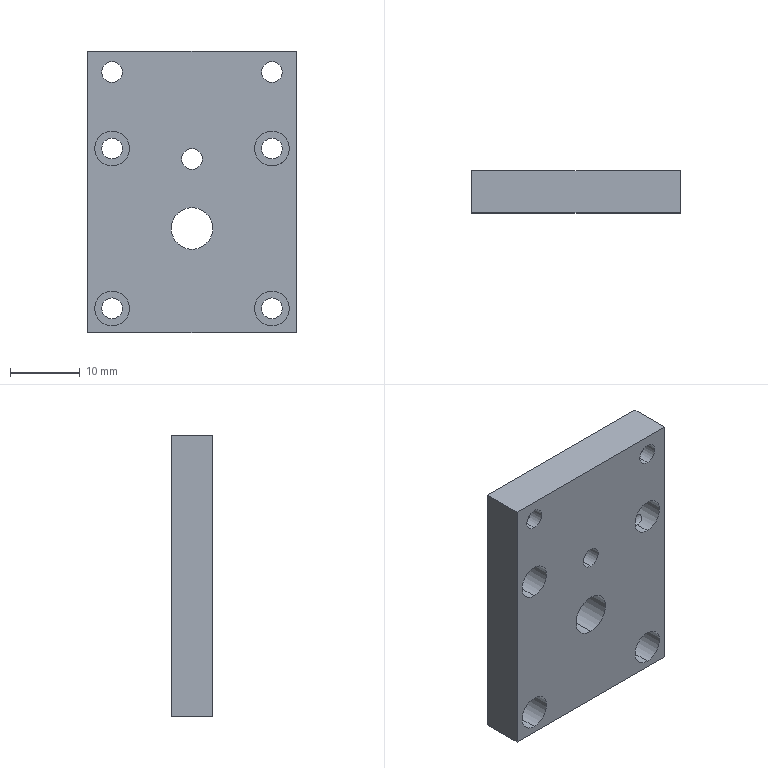Part | SolidWorks | features Cut 3, ICE 3, FlatPattern 1, HoleWzd 1, SMBaseFlange 1, SheetMetal 1 | 1 solid | 48 faces | box 30 x 6 x 40.5 mm | volume 6447 mm3 | cylinder 32 | plane 12 | cone 4 | commonest cylinder face diameters 3 x14 5 x12 2.5 x4 6 x2
STEP:
#1=CARTESIAN_POINT('',(6.749,-3.,3.));
#2=VERTEX_POINT('',#1);
#3=CARTESIAN_POINT('',(7.5,-3.,1.75));
#4=VERTEX_POINT('',#3);
#5=CARTESIAN_POINT('',(7.5,-3.,1.75));
#6=DIRECTION('',(0.515,0.,-0.8572));
#7=VECTOR('',#6,1000.);
#8=LINE('',#5,#7);
#9=EDGE_CURVE('',#2,#4,#8,.T.);
#10=ORIENTED_EDGE('',*,*,#9,.F.);
#11=CARTESIAN_POINT('',(7.5,-3.,4.25));
#12=VERTEX_POINT('',#11);
#13=CARTESIAN_POINT('',(7.5,-3.,4.25));
#14=DIRECTION('',(0.515,0.,0.8572));
#15=VECTOR('',#14,1000.);
#16=LINE('',#13,#15);
#17=EDGE_CURVE('',#2,#12,#16,.T.);
#18=ORIENTED_EDGE('',*,*,#17,.T.);
#19=CARTESIAN_POINT('',(7.5,-3.,3.));
#20=DIRECTION('',(1.,0.,0.));
#21=DIRECTION('',(0.,0.,-1.));
#22=AXIS2_PLACEMENT_3D('',#19,#20,#21);
#23=CIRCLE('',#22,1.25);
#24=EDGE_CURVE('',#12,#4,#23,.T.);
#25=ORIENTED_EDGE('',*,*,#24,.T.);
#26=EDGE_LOOP('',(#10,#18,#25));
#27=FACE_OUTER_BOUND('',#26,.T.);
#28=CARTESIAN_POINT('',(7.5,-3.,3.));
#29=DIRECTION('',(1.,0.,0.));
#30=DIRECTION('',(0.,0.,-1.));
#31=AXIS2_PLACEMENT_3D('',#28,#29,#30);
#32=CONICAL_SURFACE('',#31,1.25,1.03);
#33=ADVANCED_FACE('',(#27),#32,.F.);
#34=ORIENTED_EDGE('',*,*,#24,.F.);
#35=CARTESIAN_POINT('',(10.,-3.,4.25));
#36=VERTEX_POINT('',#35);
#37=CARTESIAN_POINT('',(15.,-3.,4.25));
#38=DIRECTION('',(1.,0.,0.));
#39=VECTOR('',#38,1000.);
#40=LINE('',#37,#39);
#41=EDGE_CURVE('',#12,#36,#40,.T.);
#42=ORIENTED_EDGE('',*,*,#41,.T.);
#43=CARTESIAN_POINT('',(11.5,-4.,3.75));
#44=VERTEX_POINT('',#43);
#45=CARTESIAN_POINT('',(11.5,-4.,3.75));
#46=CARTESIAN_POINT('',(11.325,-4.,3.75));
#47=CARTESIAN_POINT('',(11.15,-3.987,3.769));
#48=CARTESIAN_POINT('',(10.815,-3.927,3.839));
#49=CARTESIAN_POINT('',(10.651,-3.88,3.893));
#50=CARTESIAN_POINT('',(10.362,-3.731,4.019));
#51=CARTESIAN_POINT('',(10.233,-3.627,4.092));
#52=CARTESIAN_POINT('',(10.051,-3.348,4.21));
#53=CARTESIAN_POINT('',(10.,-3.177,4.25));
#54=CARTESIAN_POINT('',(10.,-3.,4.25));
#55=B_SPLINE_CURVE_WITH_KNOTS('',3,(#45,#46,#47,#48,#49,#50,#51,#52,#53,#54),.UNSPECIFIED.,.F.,.F.,(4,2,2,2,4),(0.004168,0.004689,0.00521,0.005731,0.006252),.UNSPECIFIED.);
#56=EDGE_CURVE('',#44,#36,#55,.T.);
#57=ORIENTED_EDGE('',*,*,#56,.F.);
#58=CARTESIAN_POINT('',(13.,-3.,4.25));
#59=VERTEX_POINT('',#58);
#60=CARTESIAN_POINT('',(13.,-3.,4.25));
#61=CARTESIAN_POINT('',(13.,-3.176,4.25));
#62=CARTESIAN_POINT('',(12.949,-3.349,4.21));
#63=CARTESIAN_POINT('',(12.813,-3.557,4.122));
#64=CARTESIAN_POINT('',(12.758,-3.618,4.088));
#65=CARTESIAN_POINT('',(12.634,-3.724,4.021));
#66=CARTESIAN_POINT('',(12.567,-3.768,3.988));
#67=CARTESIAN_POINT('',(12.349,-3.88,3.893));
#68=CARTESIAN_POINT('',(12.187,-3.927,3.84));
#69=CARTESIAN_POINT('',(11.85,-3.987,3.769));
#70=CARTESIAN_POINT('',(11.675,-4.,3.75));
#71=CARTESIAN_POINT('',(11.5,-4.,3.75));
#72=B_SPLINE_CURVE_WITH_KNOTS('',3,(#60,#61,#62,#63,#64,#65,#66,#67,#68,#69,#70,#71),.UNSPECIFIED.,.F.,.F.,(4,2,2,2,2,4),(0.002085,0.002606,0.002866,0.003126,0.003647,0.004168),.UNSPECIFIED.);
#73=EDGE_CURVE('',#59,#44,#72,.T.);
#74=ORIENTED_EDGE('',*,*,#73,.F.);
#75=CARTESIAN_POINT('',(15.,-3.,4.25));
#76=VERTEX_POINT('',#75);
#77=CARTESIAN_POINT('',(15.,-3.,4.25));
#78=DIRECTION('',(1.,0.,0.));
#79=VECTOR('',#78,1000.);
#80=LINE('',#77,#79);
#81=EDGE_CURVE('',#59,#76,#80,.T.);
#82=ORIENTED_EDGE('',*,*,#81,.T.);
#83=CARTESIAN_POINT('',(15.,-3.,1.75));
#84=VERTEX_POINT('',#83);
#85=CARTESIAN_POINT('',(15.,-3.,3.));
#86=DIRECTION('',(1.,0.,0.));
#87=DIRECTION('',(0.,0.,-1.));
#88=AXIS2_PLACEMENT_3D('',#85,#86,#87);
#89=CIRCLE('',#88,1.25);
#90=EDGE_CURVE('',#76,#84,#89,.T.);
#91=ORIENTED_EDGE('',*,*,#90,.T.);
#92=CARTESIAN_POINT('',(15.,-3.,1.75));
#93=DIRECTION('',(1.,0.,0.));
#94=VECTOR('',#93,1000.);
#95=LINE('',#92,#94);
#96=EDGE_CURVE('',#4,#84,#95,.T.);
#97=ORIENTED_EDGE('',*,*,#96,.F.);
#98=EDGE_LOOP('',(#34,#42,#57,#74,#82,#91,#97));
#99=FACE_OUTER_BOUND('',#98,.T.);
#100=CARTESIAN_POINT('',(15.,-3.,3.));
#101=DIRECTION('',(1.,0.,0.));
#102=DIRECTION('',(0.,0.,-1.));
#103=AXIS2_PLACEMENT_3D('',#100,#101,#102);
#104=CYLINDRICAL_SURFACE('',#103,1.25);
#105=ADVANCED_FACE('',(#99),#104,.F.);
#106=CARTESIAN_POINT('',(7.5,-3.,-5.25));
#107=VERTEX_POINT('',#106);
#108=CARTESIAN_POINT('',(7.5,-3.,-7.75));
#109=VERTEX_POINT('',#108);
#110=CARTESIAN_POINT('',(7.5,-3.,-6.5));
#111=DIRECTION('',(1.,0.,0.));
#112=DIRECTION('',(0.,0.,-1.));
#113=AXIS2_PLACEMENT_3D('',#110,#111,#112);
#114=CIRCLE('',#113,1.25);
#115=EDGE_CURVE('',#107,#109,#114,.T.);
#116=ORIENTED_EDGE('',*,*,#115,.F.);
#117=CARTESIAN_POINT('',(15.,-3.,-5.25));
#118=VERTEX_POINT('',#117);
#119=CARTESIAN_POINT('',(15.,-3.,-5.25));
#120=DIRECTION('',(1.,0.,0.));
#121=VECTOR('',#120,1000.);
#122=LINE('',#119,#121);
#123=EDGE_CURVE('',#107,#118,#122,.T.);
#124=ORIENTED_EDGE('',*,*,#123,.T.);
#125=CARTESIAN_POINT('',(15.,-3.,-7.75));
#126=VERTEX_POINT('',#125);
#127=CARTESIAN_POINT('',(15.,-3.,-6.5));
#128=DIRECTION('',(1.,0.,0.));
#129=DIRECTION('',(0.,0.,-1.));
#130=AXIS2_PLACEMENT_3D('',#127,#128,#129);
#131=CIRCLE('',#130,1.25);
#132=EDGE_CURVE('',#118,#126,#131,.T.);
#133=ORIENTED_EDGE('',*,*,#132,.T.);
#134=CARTESIAN_POINT('',(15.,-3.,-7.75));
#135=DIRECTION('',(1.,0.,0.));
#136=VECTOR('',#135,1000.);
#137=LINE('',#134,#136);
#138=EDGE_CURVE('',#109,#126,#137,.T.);
#139=ORIENTED_EDGE('',*,*,#138,.F.);
#140=EDGE_LOOP('',(#116,#124,#133,#139));
#141=FACE_OUTER_BOUND('',#140,.T.);
#142=CARTESIAN_POINT('',(15.,-3.,-6.5));
#143=DIRECTION('',(1.,0.,0.));
#144=DIRECTION('',(0.,0.,-1.));
#145=AXIS2_PLACEMENT_3D('',#142,#143,#144);
#146=CYLINDRICAL_SURFACE('',#145,1.25);
#147=ADVANCED_FACE('',(#141),#146,.F.);
#148=CARTESIAN_POINT('',(6.749,-3.,-6.5));
#149=VERTEX_POINT('',#148);
#150=CARTESIAN_POINT('',(7.5,-3.,-7.75));
#151=DIRECTION('',(0.515,0.,-0.8572));
#152=VECTOR('',#151,1000.);
#153=LINE('',#150,#152);
#154=EDGE_CURVE('',#149,#109,#153,.T.);
#155=ORIENTED_EDGE('',*,*,#154,.F.);
#156=CARTESIAN_POINT('',(7.5,-3.,-5.25));
#157=DIRECTION('',(0.515,0.,0.8572));
#158=VECTOR('',#157,1000.);
#159=LINE('',#156,#158);
#160=EDGE_CURVE('',#149,#107,#159,.T.);
#161=ORIENTED_EDGE('',*,*,#160,.T.);
#162=ORIENTED_EDGE('',*,*,#115,.T.);
#163=EDGE_LOOP('',(#155,#161,#162));
#164=FACE_OUTER_BOUND('',#163,.T.);
#165=CARTESIAN_POINT('',(7.5,-3.,-6.5));
#166=DIRECTION('',(1.,0.,0.));
#167=DIRECTION('',(0.,0.,-1.));
#168=AXIS2_PLACEMENT_3D('',#165,#166,#167);
#169=CONICAL_SURFACE('',#168,1.25,1.03);
#170=ADVANCED_FACE('',(#164),#169,.F.);
#171=CARTESIAN_POINT('',(11.5,-4.,14.75));
#172=VERTEX_POINT('',#171);
#173=CARTESIAN_POINT('',(11.5,-4.,19.75));
#174=VERTEX_POINT('',#173);
#175=CARTESIAN_POINT('',(11.5,-4.,17.25));
#176=DIRECTION('',(0.,1.,0.));
#177=DIRECTION('',(0.,0.,1.));
#178=AXIS2_PLACEMENT_3D('',#175,#176,#177);
#179=CIRCLE('',#178,2.5);
#180=EDGE_CURVE('',#172,#174,#179,.T.);
#181=ORIENTED_EDGE('',*,*,#180,.F.);
#182=CARTESIAN_POINT('',(11.5,0.,14.75));
#183=VERTEX_POINT('',#182);
#184=CARTESIAN_POINT('',(11.5,-4.,14.75));
#185=DIRECTION('',(0.,1.,0.));
#186=VECTOR('',#185,1000.);
#187=LINE('',#184,#186);
#188=EDGE_CURVE('',#172,#183,#187,.T.);
#189=ORIENTED_EDGE('',*,*,#188,.T.);
#190=CARTESIAN_POINT('',(11.5,0.,19.75));
#191=VERTEX_POINT('',#190);
#192=CARTESIAN_POINT('',(11.5,0.,17.25));
#193=DIRECTION('',(0.,1.,0.));
#194=DIRECTION('',(0.,0.,1.));
#195=AXIS2_PLACEMENT_3D('',#192,#193,#194);
#196=CIRCLE('',#195,2.5);
#197=EDGE_CURVE('',#183,#191,#196,.T.);
#198=ORIENTED_EDGE('',*,*,#197,.T.);
#199=CARTESIAN_POINT('',(11.5,-4.,19.75));
#200=DIRECTION('',(0.,1.,0.));
#201=VECTOR('',#200,1000.);
#202=LINE('',#199,#201);
#203=EDGE_CURVE('',#174,#191,#202,.T.);
#204=ORIENTED_EDGE('',*,*,#203,.F.);
#205=EDGE_LOOP('',(#181,#189,#198,#204));
#206=FACE_OUTER_BOUND('',#205,.T.);
#207=CARTESIAN_POINT('',(11.5,-4.,17.25));
#208=DIRECTION('',(0.,1.,0.));
#209=DIRECTION('',(0.,0.,1.));
#210=AXIS2_PLACEMENT_3D('',#207,#208,#209);
#211=CYLINDRICAL_SURFACE('',#210,2.5);
#212=ADVANCED_FACE('',(#206),#211,.F.);
#213=CARTESIAN_POINT('',(-11.5,-4.,14.75));
#214=VERTEX_POINT('',#213);
#215=CARTESIAN_POINT('',(-11.5,-4.,19.75));
#216=VERTEX_POINT('',#215);
#217=CARTESIAN_POINT('',(-11.5,-4.,17.25));
#218=DIRECTION('',(0.,1.,0.));
#219=DIRECTION('',(0.,0.,1.));
#220=AXIS2_PLACEMENT_3D('',#217,#218,#219);
#221=CIRCLE('',#220,2.5);
#222=EDGE_CURVE('',#214,#216,#221,.T.);
#223=ORIENTED_EDGE('',*,*,#222,.F.);
#224=CARTESIAN_POINT('',(-11.5,0.,14.75));
#225=VERTEX_POINT('',#224);
#226=CARTESIAN_POINT('',(-11.5,-4.,14.75));
#227=DIRECTION('',(0.,1.,0.));
#228=VECTOR('',#227,1000.);
#229=LINE('',#226,#228);
#230=EDGE_CURVE('',#214,#225,#229,.T.);
#231=ORIENTED_EDGE('',*,*,#230,.T.);
#232=CARTESIAN_POINT('',(-11.5,0.,19.75));
#233=VERTEX_POINT('',#232);
#234=CARTESIAN_POINT('',(-11.5,0.,17.25));
#235=DIRECTION('',(0.,1.,0.));
#236=DIRECTION('',(0.,0.,1.));
#237=AXIS2_PLACEMENT_3D('',#234,#235,#236);
#238=CIRCLE('',#237,2.5);
#239=EDGE_CURVE('',#225,#233,#238,.T.);
#240=ORIENTED_EDGE('',*,*,#239,.T.);
#241=CARTESIAN_POINT('',(-11.5,-4.,19.75));
#242=DIRECTION('',(0.,1.,0.));
#243=VECTOR('',#242,1000.);
#244=LINE('',#241,#243);
#245=EDGE_CURVE('',#216,#233,#244,.T.);
#246=ORIENTED_EDGE('',*,*,#245,.F.);
#247=EDGE_LOOP('',(#223,#231,#240,#246));
#248=FACE_OUTER_BOUND('',#247,.T.);
#249=CARTESIAN_POINT('',(-11.5,-4.,17.25));
#250=DIRECTION('',(0.,1.,0.));
#251=DIRECTION('',(0.,0.,1.));
#252=AXIS2_PLACEMENT_3D('',#249,#250,#251);
#253=CYLINDRICAL_SURFACE('',#252,2.5);
#254=ADVANCED_FACE('',(#248),#253,.F.);
#255=CARTESIAN_POINT('',(11.5,-2.,-14.25));
#256=VERTEX_POINT('',#255);
#257=CARTESIAN_POINT('',(11.5,-2.,-19.25));
#258=VERTEX_POINT('',#257);
#259=CARTESIAN_POINT('',(11.5,-2.,-16.75));
#260=DIRECTION('',(0.,-1.,0.));
#261=DIRECTION('',(0.,0.,-1.));
#262=AXIS2_PLACEMENT_3D('',#259,#260,#261);
#263=CIRCLE('',#262,2.5);
#264=EDGE_CURVE('',#256,#258,#263,.T.);
#265=ORIENTED_EDGE('',*,*,#264,.F.);
#266=CARTESIAN_POINT('',(11.5,-6.,-14.25));
#267=VERTEX_POINT('',#266);
#268=CARTESIAN_POINT('',(11.5,-2.,-14.25));
#269=DIRECTION('',(0.,-1.,0.));
#270=VECTOR('',#269,1000.);
#271=LINE('',#268,#270);
#272=EDGE_CURVE('',#256,#267,#271,.T.);
#273=ORIENTED_EDGE('',*,*,#272,.T.);
#274=CARTESIAN_POINT('',(11.5,-6.,-19.25));
#275=VERTEX_POINT('',#274);
#276=CARTESIAN_POINT('',(11.5,-6.,-16.75));
#277=DIRECTION('',(0.,-1.,0.));
#278=DIRECTION('',(0.,0.,-1.));
#279=AXIS2_PLACEMENT_3D('',#276,#277,#278);
#280=CIRCLE('',#279,2.5);
#281=EDGE_CURVE('',#267,#275,#280,.T.);
#282=ORIENTED_EDGE('',*,*,#281,.T.);
#283=CARTESIAN_POINT('',(11.5,-2.,-19.25));
#284=DIRECTION('',(0.,-1.,0.));
#285=VECTOR('',#284,1000.);
#286=LINE('',#283,#285);
#287=EDGE_CURVE('',#258,#275,#286,.T.);
#288=ORIENTED_EDGE('',*,*,#287,.F.);
#289=EDGE_LOOP('',(#265,#273,#282,#288));
#290=FACE_OUTER_BOUND('',#289,.T.);
#291=CARTESIAN_POINT('',(11.5,-2.,-16.75));
#292=DIRECTION('',(0.,-1.,0.));
#293=DIRECTION('',(0.,0.,-1.));
#294=AXIS2_PLACEMENT_3D('',#291,#292,#293);
#295=CYLINDRICAL_SURFACE('',#294,2.5);
#296=ADVANCED_FACE('',(#290),#295,.F.);
#297=CARTESIAN_POINT('',(11.5,-2.,8.75));
#298=VERTEX_POINT('',#297);
#299=CARTESIAN_POINT('',(11.5,-2.,3.75));
#300=VERTEX_POINT('',#299);
#301=CARTESIAN_POINT('',(11.5,-2.,6.25));
#302=DIRECTION('',(0.,-1.,0.));
#303=DIRECTION('',(0.,0.,-1.));
#304=AXIS2_PLACEMENT_3D('',#301,#302,#303);
#305=CIRCLE('',#304,2.5);
#306=EDGE_CURVE('',#298,#300,#305,.T.);
#307=ORIENTED_EDGE('',*,*,#306,.F.);
#308=CARTESIAN_POINT('',(11.5,-6.,8.75));
#309=VERTEX_POINT('',#308);
#310=CARTESIAN_POINT('',(11.5,-2.,8.75));
#311=DIRECTION('',(0.,-1.,0.));
#312=VECTOR('',#311,1000.);
#313=LINE('',#310,#312);
#314=EDGE_CURVE('',#298,#309,#313,.T.);
#315=ORIENTED_EDGE('',*,*,#314,.T.);
#316=CARTESIAN_POINT('',(11.5,-6.,3.75));
#317=VERTEX_POINT('',#316);
#318=CARTESIAN_POINT('',(11.5,-6.,6.25));
#319=DIRECTION('',(0.,-1.,0.));
#320=DIRECTION('',(0.,0.,-1.));
#321=AXIS2_PLACEMENT_3D('',#318,#319,#320);
#322=CIRCLE('',#321,2.5);
#323=EDGE_CURVE('',#309,#317,#322,.T.);
#324=ORIENTED_EDGE('',*,*,#323,.T.);
#325=CARTESIAN_POINT('',(11.5,-2.,3.75));
#326=DIRECTION('',(0.,-1.,0.));
#327=VECTOR('',#326,1000.);
#328=LINE('',#325,#327);
#329=EDGE_CURVE('',#44,#317,#328,.T.);
#330=ORIENTED_EDGE('',*,*,#329,.F.);
#331=ORIENTED_EDGE('',*,*,#56,.T.);
#332=CARTESIAN_POINT('',(10.,-3.,4.25));
#333=CARTESIAN_POINT('',(10.,-2.823,4.25));
#334=CARTESIAN_POINT('',(10.051,-2.652,4.21));
#335=CARTESIAN_POINT('',(10.233,-2.373,4.092));
#336=CARTESIAN_POINT('',(10.361,-2.269,4.019));
#337=CARTESIAN_POINT('',(10.65,-2.121,3.894));
#338=CARTESIAN_POINT('',(10.813,-2.073,3.84));
#339=CARTESIAN_POINT('',(11.148,-2.013,3.769));
#340=CARTESIAN_POINT('',(11.324,-2.,3.75));
#341=CARTESIAN_POINT('',(11.5,-2.,3.75));
#342=B_SPLINE_CURVE_WITH_KNOTS('',3,(#332,#333,#334,#335,#336,#337,#338,#339,#340,#341),.UNSPECIFIED.,.F.,.F.,(4,2,2,2,4),(0.006252,0.006771,0.007291,0.007811,0.008331),.UNSPECIFIED.);
#343=EDGE_CURVE('',#36,#300,#342,.T.);
#344=ORIENTED_EDGE('',*,*,#343,.T.);
#345=EDGE_LOOP('',(#307,#315,#324,#330,#331,#344));
#346=FACE_OUTER_BOUND('',#345,.T.);
#347=CARTESIAN_POINT('',(11.5,-2.,6.25));
#348=DIRECTION('',(0.,-1.,0.));
#349=DIRECTION('',(0.,0.,-1.));
#350=AXIS2_PLACEMENT_3D('',#347,#348,#349);
#351=CYLINDRICAL_SURFACE('',#350,2.5);
#352=ADVANCED_FACE('',(#346),#351,.F.);
#353=CARTESIAN_POINT('',(-11.5,-2.,8.75));
#354=VERTEX_POINT('',#353);
#355=CARTESIAN_POINT('',(-11.5,-2.,3.75));
#356=VERTEX_POINT('',#355);
#357=CARTESIAN_POINT('',(-11.5,-2.,6.25));
#358=DIRECTION('',(0.,-1.,0.));
#359=DIRECTION('',(0.,0.,-1.));
#360=AXIS2_PLACEMENT_3D('',#357,#358,#359);
#361=CIRCLE('',#360,2.5);
#362=EDGE_CURVE('',#354,#356,#361,.T.);
#363=ORIENTED_EDGE('',*,*,#362,.F.);
#364=CARTESIAN_POINT('',(-11.5,-6.,8.75));
#365=VERTEX_POINT('',#364);
#366=CARTESIAN_POINT('',(-11.5,-2.,8.75));
#367=DIRECTION('',(0.,-1.,0.));
#368=VECTOR('',#367,1000.);
#369=LINE('',#366,#368);
#370=EDGE_CURVE('',#354,#365,#369,.T.);
#371=ORIENTED_EDGE('',*,*,#370,.T.);
#372=CARTESIAN_POINT('',(-11.5,-6.,3.75));
#373=VERTEX_POINT('',#372);
#374=CARTESIAN_POINT('',(-11.5,-6.,6.25));
#375=DIRECTION('',(0.,-1.,0.));
#376=DIRECTION('',(0.,0.,-1.));
#377=AXIS2_PLACEMENT_3D('',#374,#375,#376);
#378=CIRCLE('',#377,2.5);
#379=EDGE_CURVE('',#365,#373,#378,.T.);
#380=ORIENTED_EDGE('',*,*,#379,.T.);
#381=CARTESIAN_POINT('',(-11.5,-2.,3.75));
#382=DIRECTION('',(0.,-1.,0.));
#383=VECTOR('',#382,1000.);
#384=LINE('',#381,#383);
#385=EDGE_CURVE('',#356,#373,#384,.T.);
#386=ORIENTED_EDGE('',*,*,#385,.F.);
#387=EDGE_LOOP('',(#363,#371,#380,#386));
#388=FACE_OUTER_BOUND('',#387,.T.);
#389=CARTESIAN_POINT('',(-11.5,-2.,6.25));
#390=DIRECTION('',(0.,-1.,0.));
#391=DIRECTION('',(0.,0.,-1.));
#392=AXIS2_PLACEMENT_3D('',#389,#390,#391);
#393=CYLINDRICAL_SURFACE('',#392,2.5);
#394=ADVANCED_FACE('',(#388),#393,.F.);
#395=CARTESIAN_POINT('',(-11.5,-2.,-14.25));
#396=VERTEX_POINT('',#395);
#397=CARTESIAN_POINT('',(-11.5,-2.,-19.25));
#398=VERTEX_POINT('',#397);
#399=CARTESIAN_POINT('',(-11.5,-2.,-16.75));
#400=DIRECTION('',(0.,-1.,0.));
#401=DIRECTION('',(0.,0.,-1.));
#402=AXIS2_PLACEMENT_3D('',#399,#400,#401);
#403=CIRCLE('',#402,2.5);
#404=EDGE_CURVE('',#396,#398,#403,.T.);
#405=ORIENTED_EDGE('',*,*,#404,.F.);
#406=CARTESIAN_POINT('',(-11.5,-6.,-14.25));
#407=VERTEX_POINT('',#406);
#408=CARTESIAN_POINT('',(-11.5,-2.,-14.25));
#409=DIRECTION('',(0.,-1.,0.));
#410=VECTOR('',#409,1000.);
#411=LINE('',#408,#410);
#412=EDGE_CURVE('',#396,#407,#411,.T.);
#413=ORIENTED_EDGE('',*,*,#412,.T.);
#414=CARTESIAN_POINT('',(-11.5,-6.,-19.25));
#415=VERTEX_POINT('',#414);
#416=CARTESIAN_POINT('',(-11.5,-6.,-16.75));
#417=DIRECTION('',(0.,-1.,0.));
#418=DIRECTION('',(0.,0.,-1.));
#419=AXIS2_PLACEMENT_3D('',#416,#417,#418);
#420=CIRCLE('',#419,2.5);
#421=EDGE_CURVE('',#407,#415,#420,.T.);
#422=ORIENTED_EDGE('',*,*,#421,.T.);
#423=CARTESIAN_POINT('',(-11.5,-2.,-19.25));
#424=DIRECTION('',(0.,-1.,0.));
#425=VECTOR('',#424,1000.);
#426=LINE('',#423,#425);
#427=EDGE_CURVE('',#398,#415,#426,.T.);
#428=ORIENTED_EDGE('',*,*,#427,.F.);
#429=EDGE_LOOP('',(#405,#413,#422,#428));
#430=FACE_OUTER_BOUND('',#429,.T.);
#431=CARTESIAN_POINT('',(-11.5,-2.,-16.75));
#432=DIRECTION('',(0.,-1.,0.));
#433=DIRECTION('',(0.,0.,-1.));
#434=AXIS2_PLACEMENT_3D('',#431,#432,#433);
#435=CYLINDRICAL_SURFACE('',#434,2.5);
#436=ADVANCED_FACE('',(#430),#435,.F.);
#437=CARTESIAN_POINT('',(0.,0.,-2.25));
#438=VERTEX_POINT('',#437);
#439=CARTESIAN_POINT('',(0.,0.,-8.25));
#440=VERTEX_POINT('',#439);
#441=CARTESIAN_POINT('',(0.,0.,-5.25));
#442=DIRECTION('',(0.,-1.,0.));
#443=DIRECTION('',(0.,0.,-1.));
#444=AXIS2_PLACEMENT_3D('',#441,#442,#443);
#445=CIRCLE('',#444,3.);
#446=EDGE_CURVE('',#438,#440,#445,.T.);
#447=ORIENTED_EDGE('',*,*,#446,.F.);
#448=CARTESIAN_POINT('',(0.,-6.,-2.25));
#449=VERTEX_POINT('',#448);
#450=CARTESIAN_POINT('',(0.,0.,-2.25));
#451=DIRECTION('',(0.,-1.,0.));
#452=VECTOR('',#451,1000.);
#453=LINE('',#450,#452);
#454=EDGE_CURVE('',#438,#449,#453,.T.);
#455=ORIENTED_EDGE('',*,*,#454,.T.);
#456=CARTESIAN_POINT('',(0.,-6.,-8.25));
#457=VERTEX_POINT('',#456);
#458=CARTESIAN_POINT('',(0.,-6.,-5.25));
#459=DIRECTION('',(0.,-1.,0.));
#460=DIRECTION('',(0.,0.,-1.));
#461=AXIS2_PLACEMENT_3D('',#458,#459,#460);
#462=CIRCLE('',#461,3.);
#463=EDGE_CURVE('',#449,#457,#462,.T.);
#464=ORIENTED_EDGE('',*,*,#463,.T.);
#465=CARTESIAN_POINT('',(0.,0.,-8.25));
#466=DIRECTION('',(0.,-1.,0.));
#467=VECTOR('',#466,1000.);
#468=LINE('',#465,#467);
#469=EDGE_CURVE('',#440,#457,#468,.T.);
#470=ORIENTED_EDGE('',*,*,#469,.F.);
#471=EDGE_LOOP('',(#447,#455,#464,#470));
#472=FACE_OUTER_BOUND('',#471,.T.);
#473=CARTESIAN_POINT('',(0.,0.,-5.25));
#474=DIRECTION('',(0.,-1.,0.));
#475=DIRECTION('',(0.,0.,-1.));
#476=AXIS2_PLACEMENT_3D('',#473,#474,#475);
#477=CYLINDRICAL_SURFACE('',#476,3.);
#478=ADVANCED_FACE('',(#472),#477,.F.);
#479=CARTESIAN_POINT('',(0.,0.,6.25));
#480=VERTEX_POINT('',#479);
#481=CARTESIAN_POINT('',(0.,0.,3.25));
#482=VERTEX_POINT('',#481);
#483=CARTESIAN_POINT('',(0.,0.,4.75));
#484=DIRECTION('',(0.,-1.,0.));
#485=DIRECTION('',(0.,0.,-1.));
#486=AXIS2_PLACEMENT_3D('',#483,#484,#485);
#487=CIRCLE('',#486,1.5);
#488=EDGE_CURVE('',#480,#482,#487,.T.);
#489=ORIENTED_EDGE('',*,*,#488,.F.);
#490=CARTESIAN_POINT('',(0.,-6.,6.25));
#491=VERTEX_POINT('',#490);
#492=CARTESIAN_POINT('',(0.,0.,6.25));
#493=DIRECTION('',(0.,-1.,0.));
#494=VECTOR('',#493,1000.);
#495=LINE('',#492,#494);
#496=EDGE_CURVE('',#480,#491,#495,.T.);
#497=ORIENTED_EDGE('',*,*,#496,.T.);
#498=CARTESIAN_POINT('',(0.,-6.,3.25));
#499=VERTEX_POINT('',#498);
#500=CARTESIAN_POINT('',(0.,-6.,4.75));
#501=DIRECTION('',(0.,-1.,0.));
#502=DIRECTION('',(0.,0.,-1.));
#503=AXIS2_PLACEMENT_3D('',#500,#501,#502);
#504=CIRCLE('',#503,1.5);
#505=EDGE_CURVE('',#491,#499,#504,.T.);
#506=ORIENTED_EDGE('',*,*,#505,.T.);
#507=CARTESIAN_POINT('',(0.,0.,3.25));
#508=DIRECTION('',(0.,-1.,0.));
#509=VECTOR('',#508,1000.);
#510=LINE('',#507,#509);
#511=EDGE_CURVE('',#482,#499,#510,.T.);
#512=ORIENTED_EDGE('',*,*,#511,.F.);
#513=EDGE_LOOP('',(#489,#497,#506,#512));
#514=FACE_OUTER_BOUND('',#513,.T.);
#515=CARTESIAN_POINT('',(0.,0.,4.75));
#516=DIRECTION('',(0.,-1.,0.));
#517=DIRECTION('',(0.,0.,-1.));
#518=AXIS2_PLACEMENT_3D('',#515,#516,#517);
#519=CYLINDRICAL_SURFACE('',#518,1.5);
#520=ADVANCED_FACE('',(#514),#519,.F.);
#521=CARTESIAN_POINT('',(-11.5,0.,-15.25));
#522=VERTEX_POINT('',#521);
#523=CARTESIAN_POINT('',(-11.5,0.,-18.25));
#524=VERTEX_POINT('',#523);
#525=CARTESIAN_POINT('',(-11.5,0.,-16.75));
#526=DIRECTION('',(0.,-1.,0.));
#527=DIRECTION('',(0.,0.,-1.));
#528=AXIS2_PLACEMENT_3D('',#525,#526,#527);
#529=CIRCLE('',#528,1.5);
#530=EDGE_CURVE('',#522,#524,#529,.T.);
#531=ORIENTED_EDGE('',*,*,#530,.F.);
#532=CARTESIAN_POINT('',(-11.5,-2.,-15.25));
#533=VERTEX_POINT('',#532);
#534=CARTESIAN_POINT('',(-11.5,0.,-15.25));
#535=DIRECTION('',(0.,-1.,0.));
#536=VECTOR('',#535,1000.);
#537=LINE('',#534,#536);
#538=EDGE_CURVE('',#522,#533,#537,.T.);
#539=ORIENTED_EDGE('',*,*,#538,.T.);
#540=CARTESIAN_POINT('',(-11.5,-2.,-18.25));
#541=VERTEX_POINT('',#540);
#542=CARTESIAN_POINT('',(-11.5,-2.,-16.75));
#543=DIRECTION('',(0.,1.,0.));
#544=DIRECTION('',(0.,0.,-1.));
#545=AXIS2_PLACEMENT_3D('',#542,#543,#544);
#546=CIRCLE('',#545,1.5);
#547=EDGE_CURVE('',#541,#533,#546,.T.);
#548=ORIENTED_EDGE('',*,*,#547,.F.);
#549=CARTESIAN_POINT('',(-11.5,0.,-18.25));
#550=DIRECTION('',(0.,-1.,0.));
#551=VECTOR('',#550,1000.);
#552=LINE('',#549,#551);
#553=EDGE_CURVE('',#524,#541,#552,.T.);
#554=ORIENTED_EDGE('',*,*,#553,.F.);
#555=EDGE_LOOP('',(#531,#539,#548,#554));
#556=FACE_OUTER_BOUND('',#555,.T.);
#557=CARTESIAN_POINT('',(-11.5,0.,-16.75));
#558=DIRECTION('',(0.,-1.,0.));
#559=DIRECTION('',(0.,0.,-1.));
#560=AXIS2_PLACEMENT_3D('',#557,#558,#559);
#561=CYLINDRICAL_SURFACE('',#560,1.5);
#562=ADVANCED_FACE('',(#556),#561,.F.);
#563=CARTESIAN_POINT('',(-11.5,0.,7.75));
#564=VERTEX_POINT('',#563);
#565=CARTESIAN_POINT('',(-11.5,0.,4.75));
#566=VERTEX_POINT('',#565);
#567=CARTESIAN_POINT('',(-11.5,0.,6.25));
#568=DIRECTION('',(0.,-1.,0.));
#569=DIRECTION('',(0.,0.,-1.));
#570=AXIS2_PLACEMENT_3D('',#567,#568,#569);
#571=CIRCLE('',#570,1.5);
#572=EDGE_CURVE('',#564,#566,#571,.T.);
#573=ORIENTED_EDGE('',*,*,#572,.F.);
#574=CARTESIAN_POINT('',(-11.5,-2.,7.75));
#575=VERTEX_POINT('',#574);
#576=CARTESIAN_POINT('',(-11.5,0.,7.75));
#577=DIRECTION('',(0.,-1.,0.));
#578=VECTOR('',#577,1000.);
#579=LINE('',#576,#578);
#580=EDGE_CURVE('',#564,#575,#579,.T.);
#581=ORIENTED_EDGE('',*,*,#580,.T.);
#582=CARTESIAN_POINT('',(-11.5,-2.,4.75));
#583=VERTEX_POINT('',#582);
#584=CARTESIAN_POINT('',(-11.5,-2.,6.25));
#585=DIRECTION('',(0.,1.,0.));
#586=DIRECTION('',(0.,0.,-1.));
#587=AXIS2_PLACEMENT_3D('',#584,#585,#586);
#588=CIRCLE('',#587,1.5);
#589=EDGE_CURVE('',#583,#575,#588,.T.);
#590=ORIENTED_EDGE('',*,*,#589,.F.);
#591=CARTESIAN_POINT('',(-11.5,0.,4.75));
#592=DIRECTION('',(0.,-1.,0.));
#593=VECTOR('',#592,1000.);
#594=LINE('',#591,#593);
#595=EDGE_CURVE('',#566,#583,#594,.T.);
#596=ORIENTED_EDGE('',*,*,#595,.F.);
#597=EDGE_LOOP('',(#573,#581,#590,#596));
#598=FACE_OUTER_BOUND('',#597,.T.);
#599=CARTESIAN_POINT('',(-11.5,0.,6.25));
#600=DIRECTION('',(0.,-1.,0.));
#601=DIRECTION('',(0.,0.,-1.));
#602=AXIS2_PLACEMENT_3D('',#599,#600,#601);
#603=CYLINDRICAL_SURFACE('',#602,1.5);
#604=ADVANCED_FACE('',(#598),#603,.F.);
#605=CARTESIAN_POINT('',(11.5,0.,7.75));
#606=VERTEX_POINT('',#605);
#607=CARTESIAN_POINT('',(11.5,0.,4.75));
#608=VERTEX_POINT('',#607);
#609=CARTESIAN_POINT('',(11.5,0.,6.25));
#610=DIRECTION('',(0.,-1.,0.));
#611=DIRECTION('',(0.,0.,-1.));
#612=AXIS2_PLACEMENT_3D('',#609,#610,#611);
#613=CIRCLE('',#612,1.5);
#614=EDGE_CURVE('',#606,#608,#613,.T.);
#615=ORIENTED_EDGE('',*,*,#614,.F.);
#616=CARTESIAN_POINT('',(11.5,-2.,7.75));
#617=VERTEX_POINT('',#616);
#618=CARTESIAN_POINT('',(11.5,0.,7.75));
#619=DIRECTION('',(0.,-1.,0.));
#620=VECTOR('',#619,1000.);
#621=LINE('',#618,#620);
#622=EDGE_CURVE('',#606,#617,#621,.T.);
#623=ORIENTED_EDGE('',*,*,#622,.T.);
#624=CARTESIAN_POINT('',(11.5,-2.,4.75));
#625=VERTEX_POINT('',#624);
#626=CARTESIAN_POINT('',(11.5,-2.,6.25));
#627=DIRECTION('',(0.,1.,0.));
#628=DIRECTION('',(0.,0.,-1.));
#629=AXIS2_PLACEMENT_3D('',#626,#627,#628);
#630=CIRCLE('',#629,1.5);
#631=EDGE_CURVE('',#625,#617,#630,.T.);
#632=ORIENTED_EDGE('',*,*,#631,.F.);
#633=CARTESIAN_POINT('',(11.5,0.,4.75));
#634=DIRECTION('',(0.,-1.,0.));
#635=VECTOR('',#634,1000.);
#636=LINE('',#633,#635);
#637=EDGE_CURVE('',#608,#625,#636,.T.);
#638=ORIENTED_EDGE('',*,*,#637,.F.);
#639=EDGE_LOOP('',(#615,#623,#632,#638));
#640=FACE_OUTER_BOUND('',#639,.T.);
#641=CARTESIAN_POINT('',(11.5,0.,6.25));
#642=DIRECTION('',(0.,-1.,0.));
#643=DIRECTION('',(0.,0.,-1.));
#644=AXIS2_PLACEMENT_3D('',#641,#642,#643);
#645=CYLINDRICAL_SURFACE('',#644,1.5);
#646=ADVANCED_FACE('',(#640),#645,.F.);
#647=CARTESIAN_POINT('',(11.5,0.,-15.25));
#648=VERTEX_POINT('',#647);
#649=CARTESIAN_POINT('',(11.5,0.,-18.25));
#650=VERTEX_POINT('',#649);
#651=CARTESIAN_POINT('',(11.5,0.,-16.75));
#652=DIRECTION('',(0.,-1.,0.));
#653=DIRECTION('',(0.,0.,-1.));
#654=AXIS2_PLACEMENT_3D('',#651,#652,#653);
#655=CIRCLE('',#654,1.5);
#656=EDGE_CURVE('',#648,#650,#655,.T.);
#657=ORIENTED_EDGE('',*,*,#656,.F.);
#658=CARTESIAN_POINT('',(11.5,-2.,-15.25));
#659=VERTEX_POINT('',#658);
#660=CARTESIAN_POINT('',(11.5,0.,-15.25));
#661=DIRECTION('',(0.,-1.,0.));
#662=VECTOR('',#661,1000.);
#663=LINE('',#660,#662);
#664=EDGE_CURVE('',#648,#659,#663,.T.);
#665=ORIENTED_EDGE('',*,*,#664,.T.);
#666=CARTESIAN_POINT('',(11.5,-2.,-18.25));
#667=VERTEX_POINT('',#666);
#668=CARTESIAN_POINT('',(11.5,-2.,-16.75));
#669=DIRECTION('',(0.,1.,0.));
#670=DIRECTION('',(0.,0.,-1.));
#671=AXIS2_PLACEMENT_3D('',#668,#669,#670);
#672=CIRCLE('',#671,1.5);
#673=EDGE_CURVE('',#667,#659,#672,.T.);
#674=ORIENTED_EDGE('',*,*,#673,.F.);
#675=CARTESIAN_POINT('',(11.5,0.,-18.25));
#676=DIRECTION('',(0.,-1.,0.));
#677=VECTOR('',#676,1000.);
#678=LINE('',#675,#677);
#679=EDGE_CURVE('',#650,#667,#678,.T.);
#680=ORIENTED_EDGE('',*,*,#679,.F.);
#681=EDGE_LOOP('',(#657,#665,#674,#680));
#682=FACE_OUTER_BOUND('',#681,.T.);
#683=CARTESIAN_POINT('',(11.5,0.,-16.75));
#684=DIRECTION('',(0.,-1.,0.));
#685=DIRECTION('',(0.,0.,-1.));
#686=AXIS2_PLACEMENT_3D('',#683,#684,#685);
#687=CYLINDRICAL_SURFACE('',#686,1.5);
#688=ADVANCED_FACE('',(#682),#687,.F.);
#689=CARTESIAN_POINT('',(-11.5,-6.,15.75));
#690=VERTEX_POINT('',#689);
#691=CARTESIAN_POINT('',(-11.5,-6.,18.75));
#692=VERTEX_POINT('',#691);
#693=CARTESIAN_POINT('',(-11.5,-6.,17.25));
#694=DIRECTION('',(0.,1.,0.));
#695=DIRECTION('',(0.,0.,1.));
#696=AXIS2_PLACEMENT_3D('',#693,#694,#695);
#697=CIRCLE('',#696,1.5);
#698=EDGE_CURVE('',#690,#692,#697,.T.);
#699=ORIENTED_EDGE('',*,*,#698,.F.);
#700=CARTESIAN_POINT('',(-11.5,-4.,15.75));
#701=VERTEX_POINT('',#700);
#702=CARTESIAN_POINT('',(-11.5,-6.,15.75));
#703=DIRECTION('',(0.,1.,0.));
#704=VECTOR('',#703,1000.);
#705=LINE('',#702,#704);
#706=EDGE_CURVE('',#690,#701,#705,.T.);
#707=ORIENTED_EDGE('',*,*,#706,.T.);
#708=CARTESIAN_POINT('',(-11.5,-4.,18.75));
#709=VERTEX_POINT('',#708);
#710=CARTESIAN_POINT('',(-11.5,-4.,17.25));
#711=DIRECTION('',(0.,-1.,0.));
#712=DIRECTION('',(0.,0.,1.));
#713=AXIS2_PLACEMENT_3D('',#710,#711,#712);
#714=CIRCLE('',#713,1.5);
#715=EDGE_CURVE('',#709,#701,#714,.T.);
#716=ORIENTED_EDGE('',*,*,#715,.F.);
#717=CARTESIAN_POINT('',(-11.5,-6.,18.75));
#718=DIRECTION('',(0.,1.,0.));
#719=VECTOR('',#718,1000.);
#720=LINE('',#717,#719);
#721=EDGE_CURVE('',#692,#709,#720,.T.);
#722=ORIENTED_EDGE('',*,*,#721,.F.);
#723=EDGE_LOOP('',(#699,#707,#716,#722));
#724=FACE_OUTER_BOUND('',#723,.T.);
#725=CARTESIAN_POINT('',(-11.5,-6.,17.25));
#726=DIRECTION('',(0.,1.,0.));
#727=DIRECTION('',(0.,0.,1.));
#728=AXIS2_PLACEMENT_3D('',#725,#726,#727);
#729=CYLINDRICAL_SURFACE('',#728,1.5);
#730=ADVANCED_FACE('',(#724),#729,.F.);
#731=CARTESIAN_POINT('',(11.5,-6.,15.75));
#732=VERTEX_POINT('',#731);
#733=CARTESIAN_POINT('',(11.5,-6.,18.75));
#734=VERTEX_POINT('',#733);
#735=CARTESIAN_POINT('',(11.5,-6.,17.25));
#736=DIRECTION('',(0.,1.,0.));
#737=DIRECTION('',(0.,0.,1.));
#738=AXIS2_PLACEMENT_3D('',#735,#736,#737);
#739=CIRCLE('',#738,1.5);
#740=EDGE_CURVE('',#732,#734,#739,.T.);
#741=ORIENTED_EDGE('',*,*,#740,.F.);
#742=CARTESIAN_POINT('',(11.5,-4.,15.75));
#743=VERTEX_POINT('',#742);
#744=CARTESIAN_POINT('',(11.5,-6.,15.75));
#745=DIRECTION('',(0.,1.,0.));
#746=VECTOR('',#745,1000.);
#747=LINE('',#744,#746);
#748=EDGE_CURVE('',#732,#743,#747,.T.);
#749=ORIENTED_EDGE('',*,*,#748,.T.);
#750=CARTESIAN_POINT('',(11.5,-4.,18.75));
#751=VERTEX_POINT('',#750);
#752=CARTESIAN_POINT('',(11.5,-4.,17.25));
#753=DIRECTION('',(0.,-1.,0.));
#754=DIRECTION('',(0.,0.,1.));
#755=AXIS2_PLACEMENT_3D('',#752,#753,#754);
#756=CIRCLE('',#755,1.5);
#757=EDGE_CURVE('',#751,#743,#756,.T.);
#758=ORIENTED_EDGE('',*,*,#757,.F.);
#759=CARTESIAN_POINT('',(11.5,-6.,18.75));
#760=DIRECTION('',(0.,1.,0.));
#761=VECTOR('',#760,1000.);
#762=LINE('',#759,#761);
#763=EDGE_CURVE('',#734,#751,#762,.T.);
#764=ORIENTED_EDGE('',*,*,#763,.F.);
#765=EDGE_LOOP('',(#741,#749,#758,#764));
#766=FACE_OUTER_BOUND('',#765,.T.);
#767=CARTESIAN_POINT('',(11.5,-6.,17.25));
#768=DIRECTION('',(0.,1.,0.));
#769=DIRECTION('',(0.,0.,1.));
#770=AXIS2_PLACEMENT_3D('',#767,#768,#769);
#771=CYLINDRICAL_SURFACE('',#770,1.5);
#772=ADVANCED_FACE('',(#766),#771,.F.);
#773=ORIENTED_EDGE('',*,*,#748,.F.);
#774=CARTESIAN_POINT('',(11.5,-6.,17.25));
#775=DIRECTION('',(0.,1.,0.));
#776=DIRECTION('',(0.,0.,1.));
#777=AXIS2_PLACEMENT_3D('',#774,#775,#776);
#778=CIRCLE('',#777,1.5);
#779=EDGE_CURVE('',#734,#732,#778,.T.);
#780=ORIENTED_EDGE('',*,*,#779,.F.);
#781=ORIENTED_EDGE('',*,*,#763,.T.);
#782=CARTESIAN_POINT('',(11.5,-4.,17.25));
#783=DIRECTION('',(0.,-1.,0.));
#784=DIRECTION('',(0.,0.,1.));
#785=AXIS2_PLACEMENT_3D('',#782,#783,#784);
#786=CIRCLE('',#785,1.5);
#787=EDGE_CURVE('',#743,#751,#786,.T.);
#788=ORIENTED_EDGE('',*,*,#787,.F.);
#789=EDGE_LOOP('',(#773,#780,#781,#788));
#790=FACE_OUTER_BOUND('',#789,.T.);
#791=CARTESIAN_POINT('',(11.5,-6.,17.25));
#792=DIRECTION('',(0.,1.,0.));
#793=DIRECTION('',(0.,0.,1.));
#794=AXIS2_PLACEMENT_3D('',#791,#792,#793);
#795=CYLINDRICAL_SURFACE('',#794,1.5);
#796=ADVANCED_FACE('',(#790),#795,.F.);
#797=ORIENTED_EDGE('',*,*,#706,.F.);
#798=CARTESIAN_POINT('',(-11.5,-6.,17.25));
#799=DIRECTION('',(0.,1.,0.));
#800=DIRECTION('',(0.,0.,1.));
#801=AXIS2_PLACEMENT_3D('',#798,#799,#800);
#802=CIRCLE('',#801,1.5);
#803=EDGE_CURVE('',#692,#690,#802,.T.);
#804=ORIENTED_EDGE('',*,*,#803,.F.);
#805=ORIENTED_EDGE('',*,*,#721,.T.);
#806=CARTESIAN_POINT('',(-11.5,-4.,17.25));
#807=DIRECTION('',(0.,-1.,0.));
#808=DIRECTION('',(0.,0.,1.));
#809=AXIS2_PLACEMENT_3D('',#806,#807,#808);
#810=CIRCLE('',#809,1.5);
#811=EDGE_CURVE('',#701,#709,#810,.T.);
#812=ORIENTED_EDGE('',*,*,#811,.F.);
#813=EDGE_LOOP('',(#797,#804,#805,#812));
#814=FACE_OUTER_BOUND('',#813,.T.);
#815=CARTESIAN_POINT('',(-11.5,-6.,17.25));
#816=DIRECTION('',(0.,1.,0.));
#817=DIRECTION('',(0.,0.,1.));
#818=AXIS2_PLACEMENT_3D('',#815,#816,#817);
#819=CYLINDRICAL_SURFACE('',#818,1.5);
#820=ADVANCED_FACE('',(#814),#819,.F.);
#821=ORIENTED_EDGE('',*,*,#664,.F.);
#822=CARTESIAN_POINT('',(11.5,0.,-16.75));
#823=DIRECTION('',(0.,-1.,0.));
#824=DIRECTION('',(0.,0.,-1.));
#825=AXIS2_PLACEMENT_3D('',#822,#823,#824);
#826=CIRCLE('',#825,1.5);
#827=EDGE_CURVE('',#650,#648,#826,.T.);
#828=ORIENTED_EDGE('',*,*,#827,.F.);
#829=ORIENTED_EDGE('',*,*,#679,.T.);
#830=CARTESIAN_POINT('',(11.5,-2.,-16.75));
#831=DIRECTION('',(0.,1.,0.));
#832=DIRECTION('',(0.,0.,-1.));
#833=AXIS2_PLACEMENT_3D('',#830,#831,#832);
#834=CIRCLE('',#833,1.5);
#835=EDGE_CURVE('',#659,#667,#834,.T.);
#836=ORIENTED_EDGE('',*,*,#835,.F.);
#837=EDGE_LOOP('',(#821,#828,#829,#836));
#838=FACE_OUTER_BOUND('',#837,.T.);
#839=CARTESIAN_POINT('',(11.5,0.,-16.75));
#840=DIRECTION('',(0.,-1.,0.));
#841=DIRECTION('',(0.,0.,-1.));
#842=AXIS2_PLACEMENT_3D('',#839,#840,#841);
#843=CYLINDRICAL_SURFACE('',#842,1.5);
#844=ADVANCED_FACE('',(#838),#843,.F.);
#845=ORIENTED_EDGE('',*,*,#622,.F.);
#846=CARTESIAN_POINT('',(11.5,0.,6.25));
#847=DIRECTION('',(0.,-1.,0.));
#848=DIRECTION('',(0.,0.,-1.));
#849=AXIS2_PLACEMENT_3D('',#846,#847,#848);
#850=CIRCLE('',#849,1.5);
#851=EDGE_CURVE('',#608,#606,#850,.T.);
#852=ORIENTED_EDGE('',*,*,#851,.F.);
#853=ORIENTED_EDGE('',*,*,#637,.T.);
#854=CARTESIAN_POINT('',(11.5,-2.,6.25));
#855=DIRECTION('',(0.,1.,0.));
#856=DIRECTION('',(0.,0.,-1.));
#857=AXIS2_PLACEMENT_3D('',#854,#855,#856);
#858=CIRCLE('',#857,1.5);
#859=EDGE_CURVE('',#617,#625,#858,.T.);
#860=ORIENTED_EDGE('',*,*,#859,.F.);
#861=EDGE_LOOP('',(#845,#852,#853,#860));
#862=FACE_OUTER_BOUND('',#861,.T.);
#863=CARTESIAN_POINT('',(11.5,0.,6.25));
#864=DIRECTION('',(0.,-1.,0.));
#865=DIRECTION('',(0.,0.,-1.));
#866=AXIS2_PLACEMENT_3D('',#863,#864,#865);
#867=CYLINDRICAL_SURFACE('',#866,1.5);
#868=ADVANCED_FACE('',(#862),#867,.F.);
#869=ORIENTED_EDGE('',*,*,#580,.F.);
#870=CARTESIAN_POINT('',(-11.5,0.,6.25));
#871=DIRECTION('',(0.,-1.,0.));
#872=DIRECTION('',(0.,0.,-1.));
#873=AXIS2_PLACEMENT_3D('',#870,#871,#872);
#874=CIRCLE('',#873,1.5);
#875=EDGE_CURVE('',#566,#564,#874,.T.);
#876=ORIENTED_EDGE('',*,*,#875,.F.);
#877=ORIENTED_EDGE('',*,*,#595,.T.);
#878=CARTESIAN_POINT('',(-11.5,-2.,6.25));
#879=DIRECTION('',(0.,1.,0.));
#880=DIRECTION('',(0.,0.,-1.));
#881=AXIS2_PLACEMENT_3D('',#878,#879,#880);
#882=CIRCLE('',#881,1.5);
#883=EDGE_CURVE('',#575,#583,#882,.T.);
#884=ORIENTED_EDGE('',*,*,#883,.F.);
#885=EDGE_LOOP('',(#869,#876,#877,#884));
#886=FACE_OUTER_BOUND('',#885,.T.);
#887=CARTESIAN_POINT('',(-11.5,0.,6.25));
#888=DIRECTION('',(0.,-1.,0.));
#889=DIRECTION('',(0.,0.,-1.));
#890=AXIS2_PLACEMENT_3D('',#887,#888,#889);
#891=CYLINDRICAL_SURFACE('',#890,1.5);
#892=ADVANCED_FACE('',(#886),#891,.F.);
#893=ORIENTED_EDGE('',*,*,#538,.F.);
#894=CARTESIAN_POINT('',(-11.5,0.,-16.75));
#895=DIRECTION('',(0.,-1.,0.));
#896=DIRECTION('',(0.,0.,-1.));
#897=AXIS2_PLACEMENT_3D('',#894,#895,#896);
#898=CIRCLE('',#897,1.5);
#899=EDGE_CURVE('',#524,#522,#898,.T.);
#900=ORIENTED_EDGE('',*,*,#899,.F.);
#901=ORIENTED_EDGE('',*,*,#553,.T.);
#902=CARTESIAN_POINT('',(-11.5,-2.,-16.75));
#903=DIRECTION('',(0.,1.,0.));
#904=DIRECTION('',(0.,0.,-1.));
#905=AXIS2_PLACEMENT_3D('',#902,#903,#904);
#906=CIRCLE('',#905,1.5);
#907=EDGE_CURVE('',#533,#541,#906,.T.);
#908=ORIENTED_EDGE('',*,*,#907,.F.);
#909=EDGE_LOOP('',(#893,#900,#901,#908));
#910=FACE_OUTER_BOUND('',#909,.T.);
#911=CARTESIAN_POINT('',(-11.5,0.,-16.75));
#912=DIRECTION('',(0.,-1.,0.));
#913=DIRECTION('',(0.,0.,-1.));
#914=AXIS2_PLACEMENT_3D('',#911,#912,#913);
#915=CYLINDRICAL_SURFACE('',#914,1.5);
#916=ADVANCED_FACE('',(#910),#915,.F.);
#917=CARTESIAN_POINT('',(15.,-3.,3.));
#918=DIRECTION('',(1.,0.,0.));
#919=DIRECTION('',(0.,0.,-1.));
#920=AXIS2_PLACEMENT_3D('',#917,#918,#919);
#921=CIRCLE('',#920,1.25);
#922=EDGE_CURVE('',#84,#76,#921,.T.);
#923=ORIENTED_EDGE('',*,*,#922,.F.);
#924=ORIENTED_EDGE('',*,*,#90,.F.);
#925=EDGE_LOOP('',(#923,#924));
#926=FACE_BOUND('',#925,.T.);
#927=CARTESIAN_POINT('',(15.,-3.,-6.5));
#928=DIRECTION('',(1.,0.,0.));
#929=DIRECTION('',(0.,0.,-1.));
#930=AXIS2_PLACEMENT_3D('',#927,#928,#929);
#931=CIRCLE('',#930,1.25);
#932=EDGE_CURVE('',#126,#118,#931,.T.);
#933=ORIENTED_EDGE('',*,*,#932,.F.);
#934=ORIENTED_EDGE('',*,*,#132,.F.);
#935=EDGE_LOOP('',(#933,#934));
#936=FACE_BOUND('',#935,.T.);
#937=CARTESIAN_POINT('',(15.,0.,20.25));
#938=VERTEX_POINT('',#937);
#939=CARTESIAN_POINT('',(15.,0.,-20.25));
#940=VERTEX_POINT('',#939);
#941=CARTESIAN_POINT('',(15.,0.,-20.25));
#942=DIRECTION('',(0.,0.,-1.));
#943=VECTOR('',#942,1000.);
#944=LINE('',#941,#943);
#945=EDGE_CURVE('',#938,#940,#944,.T.);
#946=ORIENTED_EDGE('',*,*,#945,.F.);
#947=CARTESIAN_POINT('',(15.,-6.,20.25));
#948=VERTEX_POINT('',#947);
#949=CARTESIAN_POINT('',(15.,-6.,20.25));
#950=DIRECTION('',(0.,1.,0.));
#951=VECTOR('',#950,1000.);
#952=LINE('',#949,#951);
#953=EDGE_CURVE('',#948,#938,#952,.T.);
#954=ORIENTED_EDGE('',*,*,#953,.F.);
#955=CARTESIAN_POINT('',(15.,-6.,-20.25));
#956=VERTEX_POINT('',#955);
#957=CARTESIAN_POINT('',(15.,-6.,-20.25));
#958=DIRECTION('',(0.,0.,-1.));
#959=VECTOR('',#958,1000.);
#960=LINE('',#957,#959);
#961=EDGE_CURVE('',#948,#956,#960,.T.);
#962=ORIENTED_EDGE('',*,*,#961,.T.);
#963=CARTESIAN_POINT('',(15.,-6.,-20.25));
#964=DIRECTION('',(0.,1.,0.));
#965=VECTOR('',#964,1000.);
#966=LINE('',#963,#965);
#967=EDGE_CURVE('',#956,#940,#966,.T.);
#968=ORIENTED_EDGE('',*,*,#967,.T.);
#969=EDGE_LOOP('',(#946,#954,#962,#968));
#970=FACE_OUTER_BOUND('',#969,.T.);
#971=CARTESIAN_POINT('',(15.,-6.,-20.25));
#972=DIRECTION('',(1.,0.,0.));
#973=DIRECTION('',(0.,0.,-1.));
#974=AXIS2_PLACEMENT_3D('',#971,#972,#973);
#975=PLANE('',#974);
#976=ADVANCED_FACE('',(#926,#936,#970),#975,.T.);
#977=CARTESIAN_POINT('',(-15.,0.,20.25));
#978=VERTEX_POINT('',#977);
#979=CARTESIAN_POINT('',(-15.,0.,20.25));
#980=DIRECTION('',(1.,0.,0.));
#981=VECTOR('',#980,1000.);
#982=LINE('',#979,#981);
#983=EDGE_CURVE('',#978,#938,#982,.T.);
#984=ORIENTED_EDGE('',*,*,#983,.F.);
#985=CARTESIAN_POINT('',(-15.,-6.,20.25));
#986=VERTEX_POINT('',#985);
#987=CARTESIAN_POINT('',(-15.,-6.,20.25));
#988=DIRECTION('',(0.,1.,0.));
#989=VECTOR('',#988,1000.);
#990=LINE('',#987,#989);
#991=EDGE_CURVE('',#986,#978,#990,.T.);
#992=ORIENTED_EDGE('',*,*,#991,.F.);
#993=CARTESIAN_POINT('',(-15.,-6.,20.25));
#994=DIRECTION('',(1.,0.,0.));
#995=VECTOR('',#994,1000.);
#996=LINE('',#993,#995);
#997=EDGE_CURVE('',#986,#948,#996,.T.);
#998=ORIENTED_EDGE('',*,*,#997,.T.);
#999=ORIENTED_EDGE('',*,*,#953,.T.);
#1000=EDGE_LOOP('',(#984,#992,#998,#999));
#1001=FACE_OUTER_BOUND('',#1000,.T.);
#1002=CARTESIAN_POINT('',(-15.,-6.,20.25));
#1003=DIRECTION('',(0.,0.,1.));
#1004=DIRECTION('',(1.,0.,0.));
#1005=AXIS2_PLACEMENT_3D('',#1002,#1003,#1004);
#1006=PLANE('',#1005);
#1007=ADVANCED_FACE('',(#1001),#1006,.T.);
#1008=CARTESIAN_POINT('',(-15.,0.,-20.25));
#1009=VERTEX_POINT('',#1008);
#1010=CARTESIAN_POINT('',(-15.,0.,-20.25));
#1011=DIRECTION('',(0.,0.,1.));
#1012=VECTOR('',#1011,1000.);
#1013=LINE('',#1010,#1012);
#1014=EDGE_CURVE('',#1009,#978,#1013,.T.);
#1015=ORIENTED_EDGE('',*,*,#1014,.F.);
#1016=CARTESIAN_POINT('',(-15.,-6.,-20.25));
#1017=VERTEX_POINT('',#1016);
#1018=CARTESIAN_POINT('',(-15.,-6.,-20.25));
#1019=DIRECTION('',(0.,1.,0.));
#1020=VECTOR('',#1019,1000.);
#1021=LINE('',#1018,#1020);
#1022=EDGE_CURVE('',#1017,#1009,#1021,.T.);
#1023=ORIENTED_EDGE('',*,*,#1022,.F.);
#1024=CARTESIAN_POINT('',(-15.,-6.,-20.25));
#1025=DIRECTION('',(0.,0.,1.));
#1026=VECTOR('',#1025,1000.);
#1027=LINE('',#1024,#1026);
#1028=EDGE_CURVE('',#1017,#986,#1027,.T.);
#1029=ORIENTED_EDGE('',*,*,#1028,.T.);
#1030=ORIENTED_EDGE('',*,*,#991,.T.);
#1031=EDGE_LOOP('',(#1015,#1023,#1029,#1030));
#1032=FACE_OUTER_BOUND('',#1031,.T.);
#1033=CARTESIAN_POINT('',(-15.,-6.,-20.25));
#1034=DIRECTION('',(-1.,0.,0.));
#1035=DIRECTION('',(0.,0.,1.));
#1036=AXIS2_PLACEMENT_3D('',#1033,#1034,#1035);
#1037=PLANE('',#1036);
#1038=ADVANCED_FACE('',(#1032),#1037,.T.);
#1039=CARTESIAN_POINT('',(-15.,0.,-20.25));
#1040=DIRECTION('',(-1.,0.,0.));
#1041=VECTOR('',#1040,1000.);
#1042=LINE('',#1039,#1041);
#1043=EDGE_CURVE('',#940,#1009,#1042,.T.);
#1044=ORIENTED_EDGE('',*,*,#1043,.F.);
#1045=ORIENTED_EDGE('',*,*,#967,.F.);
#1046=CARTESIAN_POINT('',(-15.,-6.,-20.25));
#1047=DIRECTION('',(-1.,0.,0.));
#1048=VECTOR('',#1047,1000.);
#1049=LINE('',#1046,#1048);
#1050=EDGE_CURVE('',#956,#1017,#1049,.T.);
#1051=ORIENTED_EDGE('',*,*,#1050,.T.);
#1052=ORIENTED_EDGE('',*,*,#1022,.T.);
#1053=EDGE_LOOP('',(#1044,#1045,#1051,#1052));
#1054=FACE_OUTER_BOUND('',#1053,.T.);
#1055=CARTESIAN_POINT('',(-15.,-6.,-20.25));
#1056=DIRECTION('',(0.,0.,-1.));
#1057=DIRECTION('',(-1.,0.,0.));
#1058=AXIS2_PLACEMENT_3D('',#1055,#1056,#1057);
#1059=PLANE('',#1058);
#1060=ADVANCED_FACE('',(#1054),#1059,.T.);
#1061=ORIENTED_EDGE('',*,*,#803,.T.);
#1062=ORIENTED_EDGE('',*,*,#698,.T.);
#1063=EDGE_LOOP('',(#1061,#1062));
#1064=FACE_BOUND('',#1063,.T.);
#1065=ORIENTED_EDGE('',*,*,#779,.T.);
#1066=ORIENTED_EDGE('',*,*,#740,.T.);
#1067=EDGE_LOOP('',(#1065,#1066));
#1068=FACE_BOUND('',#1067,.T.);
#1069=CARTESIAN_POINT('',(11.5,-6.,6.25));
#1070=DIRECTION('',(0.,-1.,0.));
#1071=DIRECTION('',(0.,0.,-1.));
#1072=AXIS2_PLACEMENT_3D('',#1069,#1070,#1071);
#1073=CIRCLE('',#1072,2.5);
#1074=EDGE_CURVE('',#317,#309,#1073,.T.);
#1075=ORIENTED_EDGE('',*,*,#1074,.F.);
#1076=ORIENTED_EDGE('',*,*,#323,.F.);
#1077=EDGE_LOOP('',(#1075,#1076));
#1078=FACE_BOUND('',#1077,.T.);
#1079=CARTESIAN_POINT('',(-11.5,-6.,6.25));
#1080=DIRECTION('',(0.,-1.,0.));
#1081=DIRECTION('',(0.,0.,-1.));
#1082=AXIS2_PLACEMENT_3D('',#1079,#1080,#1081);
#1083=CIRCLE('',#1082,2.5);
#1084=EDGE_CURVE('',#373,#365,#1083,.T.);
#1085=ORIENTED_EDGE('',*,*,#1084,.F.);
#1086=ORIENTED_EDGE('',*,*,#379,.F.);
#1087=EDGE_LOOP('',(#1085,#1086));
#1088=FACE_BOUND('',#1087,.T.);
#1089=CARTESIAN_POINT('',(-11.5,-6.,-16.75));
#1090=DIRECTION('',(0.,-1.,0.));
#1091=DIRECTION('',(0.,0.,-1.));
#1092=AXIS2_PLACEMENT_3D('',#1089,#1090,#1091);
#1093=CIRCLE('',#1092,2.5);
#1094=EDGE_CURVE('',#415,#407,#1093,.T.);
#1095=ORIENTED_EDGE('',*,*,#1094,.F.);
#1096=ORIENTED_EDGE('',*,*,#421,.F.);
#1097=EDGE_LOOP('',(#1095,#1096));
#1098=FACE_BOUND('',#1097,.T.);
#1099=CARTESIAN_POINT('',(11.5,-6.,-16.75));
#1100=DIRECTION('',(0.,-1.,0.));
#1101=DIRECTION('',(0.,0.,-1.));
#1102=AXIS2_PLACEMENT_3D('',#1099,#1100,#1101);
#1103=CIRCLE('',#1102,2.5);
#1104=EDGE_CURVE('',#275,#267,#1103,.T.);
#1105=ORIENTED_EDGE('',*,*,#1104,.F.);
#1106=ORIENTED_EDGE('',*,*,#281,.F.);
#1107=EDGE_LOOP('',(#1105,#1106));
#1108=FACE_BOUND('',#1107,.T.);
#1109=CARTESIAN_POINT('',(0.,-6.,-5.25));
#1110=DIRECTION('',(0.,-1.,0.));
#1111=DIRECTION('',(0.,0.,-1.));
#1112=AXIS2_PLACEMENT_3D('',#1109,#1110,#1111);
#1113=CIRCLE('',#1112,3.);
#1114=EDGE_CURVE('',#457,#449,#1113,.T.);
#1115=ORIENTED_EDGE('',*,*,#1114,.F.);
#1116=ORIENTED_EDGE('',*,*,#463,.F.);
#1117=EDGE_LOOP('',(#1115,#1116));
#1118=FACE_BOUND('',#1117,.T.);
#1119=CARTESIAN_POINT('',(0.,-6.,4.75));
#1120=DIRECTION('',(0.,-1.,0.));
#1121=DIRECTION('',(0.,0.,-1.));
#1122=AXIS2_PLACEMENT_3D('',#1119,#1120,#1121);
#1123=CIRCLE('',#1122,1.5);
#1124=EDGE_CURVE('',#499,#491,#1123,.T.);
#1125=ORIENTED_EDGE('',*,*,#1124,.F.);
#1126=ORIENTED_EDGE('',*,*,#505,.F.);
#1127=EDGE_LOOP('',(#1125,#1126));
#1128=FACE_BOUND('',#1127,.T.);
#1129=ORIENTED_EDGE('',*,*,#961,.F.);
#1130=ORIENTED_EDGE('',*,*,#997,.F.);
#1131=ORIENTED_EDGE('',*,*,#1028,.F.);
#1132=ORIENTED_EDGE('',*,*,#1050,.F.);
#1133=EDGE_LOOP('',(#1129,#1130,#1131,#1132));
#1134=FACE_OUTER_BOUND('',#1133,.T.);
#1135=CARTESIAN_POINT('',(0.,-6.,0.));
#1136=DIRECTION('',(0.,1.,0.));
#1137=DIRECTION('',(0.,0.,1.));
#1138=AXIS2_PLACEMENT_3D('',#1135,#1136,#1137);
#1139=PLANE('',#1138);
#1140=ADVANCED_FACE('',(#1064,#1068,#1078,#1088,#1098,#1108,#1118,#1128,#1134),#1139,.F.);
#1141=CARTESIAN_POINT('',(-11.5,0.,17.25));
#1142=DIRECTION('',(0.,1.,0.));
#1143=DIRECTION('',(0.,0.,1.));
#1144=AXIS2_PLACEMENT_3D('',#1141,#1142,#1143);
#1145=CIRCLE('',#1144,2.5);
#1146=EDGE_CURVE('',#233,#225,#1145,.T.);
#1147=ORIENTED_EDGE('',*,*,#1146,.F.);
#1148=ORIENTED_EDGE('',*,*,#239,.F.);
#1149=EDGE_LOOP('',(#1147,#1148));
#1150=FACE_BOUND('',#1149,.T.);
#1151=CARTESIAN_POINT('',(11.5,0.,17.25));
#1152=DIRECTION('',(0.,1.,0.));
#1153=DIRECTION('',(0.,0.,1.));
#1154=AXIS2_PLACEMENT_3D('',#1151,#1152,#1153);
#1155=CIRCLE('',#1154,2.5);
#1156=EDGE_CURVE('',#191,#183,#1155,.T.);
#1157=ORIENTED_EDGE('',*,*,#1156,.F.);
#1158=ORIENTED_EDGE('',*,*,#197,.F.);
#1159=EDGE_LOOP('',(#1157,#1158));
#1160=FACE_BOUND('',#1159,.T.);
#1161=ORIENTED_EDGE('',*,*,#899,.T.);
#1162=ORIENTED_EDGE('',*,*,#530,.T.);
#1163=EDGE_LOOP('',(#1161,#1162));
#1164=FACE_BOUND('',#1163,.T.);
#1165=ORIENTED_EDGE('',*,*,#875,.T.);
#1166=ORIENTED_EDGE('',*,*,#572,.T.);
#1167=EDGE_LOOP('',(#1165,#1166));
#1168=FACE_BOUND('',#1167,.T.);
#1169=ORIENTED_EDGE('',*,*,#851,.T.);
#1170=ORIENTED_EDGE('',*,*,#614,.T.);
#1171=EDGE_LOOP('',(#1169,#1170));
#1172=FACE_BOUND('',#1171,.T.);
#1173=CARTESIAN_POINT('',(0.,0.,-5.25));
#1174=DIRECTION('',(0.,-1.,0.));
#1175=DIRECTION('',(0.,0.,-1.));
#1176=AXIS2_PLACEMENT_3D('',#1173,#1174,#1175);
#1177=CIRCLE('',#1176,3.);
#1178=EDGE_CURVE('',#440,#438,#1177,.T.);
#1179=ORIENTED_EDGE('',*,*,#1178,.T.);
#1180=ORIENTED_EDGE('',*,*,#446,.T.);
#1181=EDGE_LOOP('',(#1179,#1180));
#1182=FACE_BOUND('',#1181,.T.);
#1183=CARTESIAN_POINT('',(0.,0.,4.75));
#1184=DIRECTION('',(0.,-1.,0.));
#1185=DIRECTION('',(0.,0.,-1.));
#1186=AXIS2_PLACEMENT_3D('',#1183,#1184,#1185);
#1187=CIRCLE('',#1186,1.5);
#1188=EDGE_CURVE('',#482,#480,#1187,.T.);
#1189=ORIENTED_EDGE('',*,*,#1188,.T.);
#1190=ORIENTED_EDGE('',*,*,#488,.T.);
#1191=EDGE_LOOP('',(#1189,#1190));
#1192=FACE_BOUND('',#1191,.T.);
#1193=ORIENTED_EDGE('',*,*,#827,.T.);
#1194=ORIENTED_EDGE('',*,*,#656,.T.);
#1195=EDGE_LOOP('',(#1193,#1194));
#1196=FACE_BOUND('',#1195,.T.);
#1197=ORIENTED_EDGE('',*,*,#945,.T.);
#1198=ORIENTED_EDGE('',*,*,#1043,.T.);
#1199=ORIENTED_EDGE('',*,*,#1014,.T.);
#1200=ORIENTED_EDGE('',*,*,#983,.T.);
#1201=EDGE_LOOP('',(#1197,#1198,#1199,#1200));
#1202=FACE_OUTER_BOUND('',#1201,.T.);
#1203=CARTESIAN_POINT('',(0.,0.,0.));
#1204=DIRECTION('',(0.,1.,0.));
#1205=DIRECTION('',(0.,0.,1.));
#1206=AXIS2_PLACEMENT_3D('',#1203,#1204,#1205);
#1207=PLANE('',#1206);
#1208=ADVANCED_FACE('',(#1150,#1160,#1164,#1168,#1172,#1182,#1192,#1196,#1202),#1207,.T.);
#1209=ORIENTED_EDGE('',*,*,#496,.F.);
#1210=ORIENTED_EDGE('',*,*,#1188,.F.);
#1211=ORIENTED_EDGE('',*,*,#511,.T.);
#1212=ORIENTED_EDGE('',*,*,#1124,.T.);
#1213=EDGE_LOOP('',(#1209,#1210,#1211,#1212));
#1214=FACE_OUTER_BOUND('',#1213,.T.);
#1215=CARTESIAN_POINT('',(0.,0.,4.75));
#1216=DIRECTION('',(0.,-1.,0.));
#1217=DIRECTION('',(0.,0.,-1.));
#1218=AXIS2_PLACEMENT_3D('',#1215,#1216,#1217);
#1219=CYLINDRICAL_SURFACE('',#1218,1.5);
#1220=ADVANCED_FACE('',(#1214),#1219,.F.);
#1221=ORIENTED_EDGE('',*,*,#454,.F.);
#1222=ORIENTED_EDGE('',*,*,#1178,.F.);
#1223=ORIENTED_EDGE('',*,*,#469,.T.);
#1224=ORIENTED_EDGE('',*,*,#1114,.T.);
#1225=EDGE_LOOP('',(#1221,#1222,#1223,#1224));
#1226=FACE_OUTER_BOUND('',#1225,.T.);
#1227=CARTESIAN_POINT('',(0.,0.,-5.25));
#1228=DIRECTION('',(0.,-1.,0.));
#1229=DIRECTION('',(0.,0.,-1.));
#1230=AXIS2_PLACEMENT_3D('',#1227,#1228,#1229);
#1231=CYLINDRICAL_SURFACE('',#1230,3.);
#1232=ADVANCED_FACE('',(#1226),#1231,.F.);
#1233=CARTESIAN_POINT('',(-11.5,-2.,-16.75));
#1234=DIRECTION('',(0.,-1.,0.));
#1235=DIRECTION('',(0.,0.,-1.));
#1236=AXIS2_PLACEMENT_3D('',#1233,#1234,#1235);
#1237=CIRCLE('',#1236,2.5);
#1238=EDGE_CURVE('',#398,#396,#1237,.T.);
#1239=ORIENTED_EDGE('',*,*,#1238,.T.);
#1240=ORIENTED_EDGE('',*,*,#404,.T.);
#1241=EDGE_LOOP('',(#1239,#1240));
#1242=FACE_OUTER_BOUND('',#1241,.T.);
#1243=ORIENTED_EDGE('',*,*,#547,.T.);
#1244=ORIENTED_EDGE('',*,*,#907,.T.);
#1245=EDGE_LOOP('',(#1243,#1244));
#1246=FACE_BOUND('',#1245,.T.);
#1247=CARTESIAN_POINT('',(-11.5,-2.,-16.75));
#1248=DIRECTION('',(0.,-1.,0.));
#1249=DIRECTION('',(0.,0.,-1.));
#1250=AXIS2_PLACEMENT_3D('',#1247,#1248,#1249);
#1251=PLANE('',#1250);
#1252=ADVANCED_FACE('',(#1242,#1246),#1251,.T.);
#1253=ORIENTED_EDGE('',*,*,#412,.F.);
#1254=ORIENTED_EDGE('',*,*,#1238,.F.);
#1255=ORIENTED_EDGE('',*,*,#427,.T.);
#1256=ORIENTED_EDGE('',*,*,#1094,.T.);
#1257=EDGE_LOOP('',(#1253,#1254,#1255,#1256));
#1258=FACE_OUTER_BOUND('',#1257,.T.);
#1259=CARTESIAN_POINT('',(-11.5,-2.,-16.75));
#1260=DIRECTION('',(0.,-1.,0.));
#1261=DIRECTION('',(0.,0.,-1.));
#1262=AXIS2_PLACEMENT_3D('',#1259,#1260,#1261);
#1263=CYLINDRICAL_SURFACE('',#1262,2.5);
#1264=ADVANCED_FACE('',(#1258),#1263,.F.);
#1265=CARTESIAN_POINT('',(-11.5,-2.,6.25));
#1266=DIRECTION('',(0.,-1.,0.));
#1267=DIRECTION('',(0.,0.,-1.));
#1268=AXIS2_PLACEMENT_3D('',#1265,#1266,#1267);
#1269=CIRCLE('',#1268,2.5);
#1270=EDGE_CURVE('',#356,#354,#1269,.T.);
#1271=ORIENTED_EDGE('',*,*,#1270,.T.);
#1272=ORIENTED_EDGE('',*,*,#362,.T.);
#1273=EDGE_LOOP('',(#1271,#1272));
#1274=FACE_OUTER_BOUND('',#1273,.T.);
#1275=ORIENTED_EDGE('',*,*,#589,.T.);
#1276=ORIENTED_EDGE('',*,*,#883,.T.);
#1277=EDGE_LOOP('',(#1275,#1276));
#1278=FACE_BOUND('',#1277,.T.);
#1279=CARTESIAN_POINT('',(-11.5,-2.,6.25));
#1280=DIRECTION('',(0.,-1.,0.));
#1281=DIRECTION('',(0.,0.,-1.));
#1282=AXIS2_PLACEMENT_3D('',#1279,#1280,#1281);
#1283=PLANE('',#1282);
#1284=ADVANCED_FACE('',(#1274,#1278),#1283,.T.);
#1285=ORIENTED_EDGE('',*,*,#370,.F.);
#1286=ORIENTED_EDGE('',*,*,#1270,.F.);
#1287=ORIENTED_EDGE('',*,*,#385,.T.);
#1288=ORIENTED_EDGE('',*,*,#1084,.T.);
#1289=EDGE_LOOP('',(#1285,#1286,#1287,#1288));
#1290=FACE_OUTER_BOUND('',#1289,.T.);
#1291=CARTESIAN_POINT('',(-11.5,-2.,6.25));
#1292=DIRECTION('',(0.,-1.,0.));
#1293=DIRECTION('',(0.,0.,-1.));
#1294=AXIS2_PLACEMENT_3D('',#1291,#1292,#1293);
#1295=CYLINDRICAL_SURFACE('',#1294,2.5);
#1296=ADVANCED_FACE('',(#1290),#1295,.F.);
#1297=CARTESIAN_POINT('',(11.5,-2.,6.25));
#1298=DIRECTION('',(0.,-1.,0.));
#1299=DIRECTION('',(0.,0.,-1.));
#1300=AXIS2_PLACEMENT_3D('',#1297,#1298,#1299);
#1301=CIRCLE('',#1300,2.5);
#1302=EDGE_CURVE('',#300,#298,#1301,.T.);
#1303=ORIENTED_EDGE('',*,*,#1302,.T.);
#1304=ORIENTED_EDGE('',*,*,#306,.T.);
#1305=EDGE_LOOP('',(#1303,#1304));
#1306=FACE_OUTER_BOUND('',#1305,.T.);
#1307=ORIENTED_EDGE('',*,*,#631,.T.);
#1308=ORIENTED_EDGE('',*,*,#859,.T.);
#1309=EDGE_LOOP('',(#1307,#1308));
#1310=FACE_BOUND('',#1309,.T.);
#1311=CARTESIAN_POINT('',(11.5,-2.,6.25));
#1312=DIRECTION('',(0.,-1.,0.));
#1313=DIRECTION('',(0.,0.,-1.));
#1314=AXIS2_PLACEMENT_3D('',#1311,#1312,#1313);
#1315=PLANE('',#1314);
#1316=ADVANCED_FACE('',(#1306,#1310),#1315,.T.);
#1317=ORIENTED_EDGE('',*,*,#314,.F.);
#1318=ORIENTED_EDGE('',*,*,#1302,.F.);
#1319=CARTESIAN_POINT('',(11.5,-2.,3.75));
#1320=CARTESIAN_POINT('',(11.676,-2.,3.75));
#1321=CARTESIAN_POINT('',(11.848,-2.013,3.768));
#1322=CARTESIAN_POINT('',(12.185,-2.073,3.84));
#1323=CARTESIAN_POINT('',(12.348,-2.12,3.893));
#1324=CARTESIAN_POINT('',(12.566,-2.232,3.987));
#1325=CARTESIAN_POINT('',(12.635,-2.277,4.021));
#1326=CARTESIAN_POINT('',(12.758,-2.382,4.088));
#1327=CARTESIAN_POINT('',(12.813,-2.444,4.122));
#1328=CARTESIAN_POINT('',(12.948,-2.651,4.21));
#1329=CARTESIAN_POINT('',(13.,-2.824,4.25));
#1330=CARTESIAN_POINT('',(13.,-3.,4.25));
#1331=B_SPLINE_CURVE_WITH_KNOTS('',3,(#1319,#1320,#1321,#1322,#1323,#1324,#1325,#1326,#1327,#1328,#1329,#1330),.UNSPECIFIED.,.F.,.F.,(4,2,2,2,2,4),(0.,0.0005213,0.001043,0.001303,0.001564,0.002085),.UNSPECIFIED.);
#1332=EDGE_CURVE('',#300,#59,#1331,.T.);
#1333=ORIENTED_EDGE('',*,*,#1332,.T.);
#1334=ORIENTED_EDGE('',*,*,#73,.T.);
#1335=ORIENTED_EDGE('',*,*,#329,.T.);
#1336=ORIENTED_EDGE('',*,*,#1074,.T.);
#1337=EDGE_LOOP('',(#1317,#1318,#1333,#1334,#1335,#1336));
#1338=FACE_OUTER_BOUND('',#1337,.T.);
#1339=CARTESIAN_POINT('',(11.5,-2.,6.25));
#1340=DIRECTION('',(0.,-1.,0.));
#1341=DIRECTION('',(0.,0.,-1.));
#1342=AXIS2_PLACEMENT_3D('',#1339,#1340,#1341);
#1343=CYLINDRICAL_SURFACE('',#1342,2.5);
#1344=ADVANCED_FACE('',(#1338),#1343,.F.);
#1345=CARTESIAN_POINT('',(11.5,-2.,-16.75));
#1346=DIRECTION('',(0.,-1.,0.));
#1347=DIRECTION('',(0.,0.,-1.));
#1348=AXIS2_PLACEMENT_3D('',#1345,#1346,#1347);
#1349=CIRCLE('',#1348,2.5);
#1350=EDGE_CURVE('',#258,#256,#1349,.T.);
#1351=ORIENTED_EDGE('',*,*,#1350,.T.);
#1352=ORIENTED_EDGE('',*,*,#264,.T.);
#1353=EDGE_LOOP('',(#1351,#1352));
#1354=FACE_OUTER_BOUND('',#1353,.T.);
#1355=ORIENTED_EDGE('',*,*,#673,.T.);
#1356=ORIENTED_EDGE('',*,*,#835,.T.);
#1357=EDGE_LOOP('',(#1355,#1356));
#1358=FACE_BOUND('',#1357,.T.);
#1359=CARTESIAN_POINT('',(11.5,-2.,-16.75));
#1360=DIRECTION('',(0.,-1.,0.));
#1361=DIRECTION('',(0.,0.,-1.));
#1362=AXIS2_PLACEMENT_3D('',#1359,#1360,#1361);
#1363=PLANE('',#1362);
#1364=ADVANCED_FACE('',(#1354,#1358),#1363,.T.);
#1365=ORIENTED_EDGE('',*,*,#272,.F.);
#1366=ORIENTED_EDGE('',*,*,#1350,.F.);
#1367=ORIENTED_EDGE('',*,*,#287,.T.);
#1368=ORIENTED_EDGE('',*,*,#1104,.T.);
#1369=EDGE_LOOP('',(#1365,#1366,#1367,#1368));
#1370=FACE_OUTER_BOUND('',#1369,.T.);
#1371=CARTESIAN_POINT('',(11.5,-2.,-16.75));
#1372=DIRECTION('',(0.,-1.,0.));
#1373=DIRECTION('',(0.,0.,-1.));
#1374=AXIS2_PLACEMENT_3D('',#1371,#1372,#1373);
#1375=CYLINDRICAL_SURFACE('',#1374,2.5);
#1376=ADVANCED_FACE('',(#1370),#1375,.F.);
#1377=CARTESIAN_POINT('',(-11.5,-4.,17.25));
#1378=DIRECTION('',(0.,1.,0.));
#1379=DIRECTION('',(0.,0.,1.));
#1380=AXIS2_PLACEMENT_3D('',#1377,#1378,#1379);
#1381=CIRCLE('',#1380,2.5);
#1382=EDGE_CURVE('',#216,#214,#1381,.T.);
#1383=ORIENTED_EDGE('',*,*,#1382,.T.);
#1384=ORIENTED_EDGE('',*,*,#222,.T.);
#1385=EDGE_LOOP('',(#1383,#1384));
#1386=FACE_OUTER_BOUND('',#1385,.T.);
#1387=ORIENTED_EDGE('',*,*,#715,.T.);
#1388=ORIENTED_EDGE('',*,*,#811,.T.);
#1389=EDGE_LOOP('',(#1387,#1388));
#1390=FACE_BOUND('',#1389,.T.);
#1391=CARTESIAN_POINT('',(-11.5,-4.,17.25));
#1392=DIRECTION('',(0.,1.,0.));
#1393=DIRECTION('',(0.,0.,1.));
#1394=AXIS2_PLACEMENT_3D('',#1391,#1392,#1393);
#1395=PLANE('',#1394);
#1396=ADVANCED_FACE('',(#1386,#1390),#1395,.T.);
#1397=ORIENTED_EDGE('',*,*,#230,.F.);
#1398=ORIENTED_EDGE('',*,*,#1382,.F.);
#1399=ORIENTED_EDGE('',*,*,#245,.T.);
#1400=ORIENTED_EDGE('',*,*,#1146,.T.);
#1401=EDGE_LOOP('',(#1397,#1398,#1399,#1400));
#1402=FACE_OUTER_BOUND('',#1401,.T.);
#1403=CARTESIAN_POINT('',(-11.5,-4.,17.25));
#1404=DIRECTION('',(0.,1.,0.));
#1405=DIRECTION('',(0.,0.,1.));
#1406=AXIS2_PLACEMENT_3D('',#1403,#1404,#1405);
#1407=CYLINDRICAL_SURFACE('',#1406,2.5);
#1408=ADVANCED_FACE('',(#1402),#1407,.F.);
#1409=CARTESIAN_POINT('',(11.5,-4.,17.25));
#1410=DIRECTION('',(0.,1.,0.));
#1411=DIRECTION('',(0.,0.,1.));
#1412=AXIS2_PLACEMENT_3D('',#1409,#1410,#1411);
#1413=CIRCLE('',#1412,2.5);
#1414=EDGE_CURVE('',#174,#172,#1413,.T.);
#1415=ORIENTED_EDGE('',*,*,#1414,.T.);
#1416=ORIENTED_EDGE('',*,*,#180,.T.);
#1417=EDGE_LOOP('',(#1415,#1416));
#1418=FACE_OUTER_BOUND('',#1417,.T.);
#1419=ORIENTED_EDGE('',*,*,#757,.T.);
#1420=ORIENTED_EDGE('',*,*,#787,.T.);
#1421=EDGE_LOOP('',(#1419,#1420));
#1422=FACE_BOUND('',#1421,.T.);
#1423=CARTESIAN_POINT('',(11.5,-4.,17.25));
#1424=DIRECTION('',(0.,1.,0.));
#1425=DIRECTION('',(0.,0.,1.));
#1426=AXIS2_PLACEMENT_3D('',#1423,#1424,#1425);
#1427=PLANE('',#1426);
#1428=ADVANCED_FACE('',(#1418,#1422),#1427,.T.);
#1429=ORIENTED_EDGE('',*,*,#188,.F.);
#1430=ORIENTED_EDGE('',*,*,#1414,.F.);
#1431=ORIENTED_EDGE('',*,*,#203,.T.);
#1432=ORIENTED_EDGE('',*,*,#1156,.T.);
#1433=EDGE_LOOP('',(#1429,#1430,#1431,#1432));
#1434=FACE_OUTER_BOUND('',#1433,.T.);
#1435=CARTESIAN_POINT('',(11.5,-4.,17.25));
#1436=DIRECTION('',(0.,1.,0.));
#1437=DIRECTION('',(0.,0.,1.));
#1438=AXIS2_PLACEMENT_3D('',#1435,#1436,#1437);
#1439=CYLINDRICAL_SURFACE('',#1438,2.5);
#1440=ADVANCED_FACE('',(#1434),#1439,.F.);
#1441=ORIENTED_EDGE('',*,*,#160,.F.);
#1442=ORIENTED_EDGE('',*,*,#154,.T.);
#1443=CARTESIAN_POINT('',(7.5,-3.,-6.5));
#1444=DIRECTION('',(1.,0.,0.));
#1445=DIRECTION('',(0.,0.,-1.));
#1446=AXIS2_PLACEMENT_3D('',#1443,#1444,#1445);
#1447=CIRCLE('',#1446,1.25);
#1448=EDGE_CURVE('',#109,#107,#1447,.T.);
#1449=ORIENTED_EDGE('',*,*,#1448,.T.);
#1450=EDGE_LOOP('',(#1441,#1442,#1449));
#1451=FACE_OUTER_BOUND('',#1450,.T.);
#1452=CARTESIAN_POINT('',(7.5,-3.,-6.5));
#1453=DIRECTION('',(1.,0.,0.));
#1454=DIRECTION('',(0.,0.,-1.));
#1455=AXIS2_PLACEMENT_3D('',#1452,#1453,#1454);
#1456=CONICAL_SURFACE('',#1455,1.25,1.03);
#1457=ADVANCED_FACE('',(#1451),#1456,.F.);
#1458=ORIENTED_EDGE('',*,*,#123,.F.);
#1459=ORIENTED_EDGE('',*,*,#1448,.F.);
#1460=ORIENTED_EDGE('',*,*,#138,.T.);
#1461=ORIENTED_EDGE('',*,*,#932,.T.);
#1462=EDGE_LOOP('',(#1458,#1459,#1460,#1461));
#1463=FACE_OUTER_BOUND('',#1462,.T.);
#1464=CARTESIAN_POINT('',(15.,-3.,-6.5));
#1465=DIRECTION('',(1.,0.,0.));
#1466=DIRECTION('',(0.,0.,-1.));
#1467=AXIS2_PLACEMENT_3D('',#1464,#1465,#1466);
#1468=CYLINDRICAL_SURFACE('',#1467,1.25);
#1469=ADVANCED_FACE('',(#1463),#1468,.F.);
#1470=ORIENTED_EDGE('',*,*,#41,.F.);
#1471=CARTESIAN_POINT('',(7.5,-3.,3.));
#1472=DIRECTION('',(1.,0.,0.));
#1473=DIRECTION('',(0.,0.,-1.));
#1474=AXIS2_PLACEMENT_3D('',#1471,#1472,#1473);
#1475=CIRCLE('',#1474,1.25);
#1476=EDGE_CURVE('',#4,#12,#1475,.T.);
#1477=ORIENTED_EDGE('',*,*,#1476,.F.);
#1478=ORIENTED_EDGE('',*,*,#96,.T.);
#1479=ORIENTED_EDGE('',*,*,#922,.T.);
#1480=ORIENTED_EDGE('',*,*,#81,.F.);
#1481=ORIENTED_EDGE('',*,*,#1332,.F.);
#1482=ORIENTED_EDGE('',*,*,#343,.F.);
#1483=EDGE_LOOP('',(#1470,#1477,#1478,#1479,#1480,#1481,#1482));
#1484=FACE_OUTER_BOUND('',#1483,.T.);
#1485=CARTESIAN_POINT('',(15.,-3.,3.));
#1486=DIRECTION('',(1.,0.,0.));
#1487=DIRECTION('',(0.,0.,-1.));
#1488=AXIS2_PLACEMENT_3D('',#1485,#1486,#1487);
#1489=CYLINDRICAL_SURFACE('',#1488,1.25);
#1490=ADVANCED_FACE('',(#1484),#1489,.F.);
#1491=ORIENTED_EDGE('',*,*,#17,.F.);
#1492=ORIENTED_EDGE('',*,*,#9,.T.);
#1493=ORIENTED_EDGE('',*,*,#1476,.T.);
#1494=EDGE_LOOP('',(#1491,#1492,#1493));
#1495=FACE_OUTER_BOUND('',#1494,.T.);
#1496=CARTESIAN_POINT('',(7.5,-3.,3.));
#1497=DIRECTION('',(1.,0.,0.));
#1498=DIRECTION('',(0.,0.,-1.));
#1499=AXIS2_PLACEMENT_3D('',#1496,#1497,#1498);
#1500=CONICAL_SURFACE('',#1499,1.25,1.03);
#1501=ADVANCED_FACE('',(#1495),#1500,.F.);
#1502=CLOSED_SHELL('',(#33,#105,#147,#170,#212,#254,#296,#352,#394,#436,#478,#520,#562,#604,#646,#688,#730,#772,#796,#820,#844,#868,#892,#916,#976,#1007,#1038,#1060,#1140,#1208,#1220,#1232,#1252,#1264,#1284,#1296,#1316,#1344,#1364,#1376,#1396,#1408,#1428,#1440,#1457,#1469,#1490,#1501));
#1503=MANIFOLD_SOLID_BREP('',#1502);
#1504=CARTESIAN_POINT('',(0.,0.,0.));
#1505=DIRECTION('',(0.,0.,1.));
#1506=DIRECTION('',(1.,0.,0.));
#1507=AXIS2_PLACEMENT_3D('',#1504,#1505,#1506);
#1508=(LENGTH_UNIT()NAMED_UNIT(*)SI_UNIT(.MILLI.,.METRE.));
#1509=UNCERTAINTY_MEASURE_WITH_UNIT(LENGTH_MEASURE(0.00001),#1508,'','');
#1510=(NAMED_UNIT(*)PLANE_ANGLE_UNIT()SI_UNIT($,.RADIAN.));
#1511=(NAMED_UNIT(*)SI_UNIT($,.STERADIAN.)SOLID_ANGLE_UNIT());
#1512=(GEOMETRIC_REPRESENTATION_CONTEXT(3)GLOBAL_UNCERTAINTY_ASSIGNED_CONTEXT((#1509))GLOBAL_UNIT_ASSIGNED_CONTEXT((#1508,#1510,#1511))REPRESENTATION_CONTEXT('',''));
#1513=ADVANCED_BREP_SHAPE_REPRESENTATION('',(#1503,#1507),#1512);